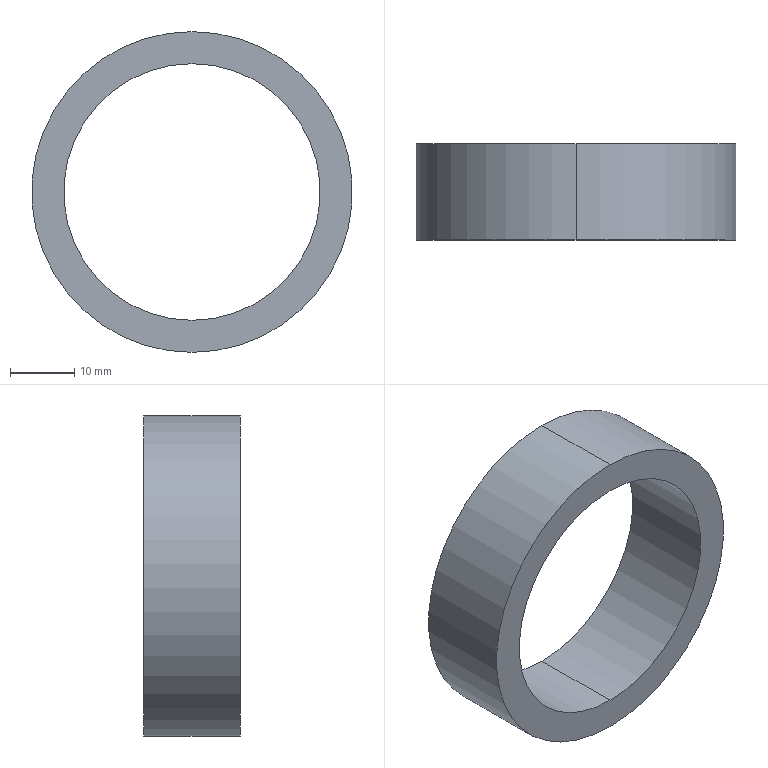Part | SolidWorks | features BaseBody 1 | 1 solid | 6 faces | box 50 x 15 x 50 mm | volume 10603 mm3 | cylinder 4 | plane 2 | commonest cylinder face diameters 40 x2 50 x2
STEP:
#1=CARTESIAN_POINT('',(0.,15.,-25.));
#2=VERTEX_POINT('',#1);
#3=CARTESIAN_POINT('',(0.,15.,25.));
#4=VERTEX_POINT('',#3);
#5=CARTESIAN_POINT('',(0.,15.,0.));
#6=DIRECTION('',(0.,-1.,0.));
#7=DIRECTION('',(0.,0.,-1.));
#8=AXIS2_PLACEMENT_3D('',#5,#6,#7);
#9=CIRCLE('',#8,25.);
#10=EDGE_CURVE('',#2,#4,#9,.T.);
#11=ORIENTED_EDGE('',*,*,#10,.T.);
#12=CARTESIAN_POINT('',(0.,0.,25.));
#13=VERTEX_POINT('',#12);
#14=CARTESIAN_POINT('',(0.,15.,25.));
#15=DIRECTION('',(0.,-1.,0.));
#16=VECTOR('',#15,1000.);
#17=LINE('',#14,#16);
#18=EDGE_CURVE('',#4,#13,#17,.T.);
#19=ORIENTED_EDGE('',*,*,#18,.T.);
#20=CARTESIAN_POINT('',(0.,0.,-25.));
#21=VERTEX_POINT('',#20);
#22=CARTESIAN_POINT('',(0.,0.,0.));
#23=DIRECTION('',(0.,1.,0.));
#24=DIRECTION('',(0.,0.,-1.));
#25=AXIS2_PLACEMENT_3D('',#22,#23,#24);
#26=CIRCLE('',#25,25.);
#27=EDGE_CURVE('',#13,#21,#26,.T.);
#28=ORIENTED_EDGE('',*,*,#27,.T.);
#29=CARTESIAN_POINT('',(0.,15.,-25.));
#30=DIRECTION('',(0.,-1.,0.));
#31=VECTOR('',#30,1000.);
#32=LINE('',#29,#31);
#33=EDGE_CURVE('',#2,#21,#32,.T.);
#34=ORIENTED_EDGE('',*,*,#33,.F.);
#35=EDGE_LOOP('',(#11,#19,#28,#34));
#36=FACE_OUTER_BOUND('',#35,.T.);
#37=CARTESIAN_POINT('',(0.,15.,0.));
#38=DIRECTION('',(0.,-1.,0.));
#39=DIRECTION('',(0.,0.,-1.));
#40=AXIS2_PLACEMENT_3D('',#37,#38,#39);
#41=CYLINDRICAL_SURFACE('',#40,25.);
#42=ADVANCED_FACE('',(#36),#41,.T.);
#43=CARTESIAN_POINT('',(0.,15.,20.));
#44=VERTEX_POINT('',#43);
#45=CARTESIAN_POINT('',(0.,15.,-20.));
#46=VERTEX_POINT('',#45);
#47=CARTESIAN_POINT('',(0.,15.,0.));
#48=DIRECTION('',(0.,-1.,0.));
#49=DIRECTION('',(0.,0.,-1.));
#50=AXIS2_PLACEMENT_3D('',#47,#48,#49);
#51=CIRCLE('',#50,20.);
#52=EDGE_CURVE('',#44,#46,#51,.T.);
#53=ORIENTED_EDGE('',*,*,#52,.F.);
#54=CARTESIAN_POINT('',(0.,0.,20.));
#55=VERTEX_POINT('',#54);
#56=CARTESIAN_POINT('',(0.,15.,20.));
#57=DIRECTION('',(0.,-1.,0.));
#58=VECTOR('',#57,1000.);
#59=LINE('',#56,#58);
#60=EDGE_CURVE('',#44,#55,#59,.T.);
#61=ORIENTED_EDGE('',*,*,#60,.T.);
#62=CARTESIAN_POINT('',(0.,0.,-20.));
#63=VERTEX_POINT('',#62);
#64=CARTESIAN_POINT('',(0.,0.,0.));
#65=DIRECTION('',(0.,-1.,0.));
#66=DIRECTION('',(0.,0.,-1.));
#67=AXIS2_PLACEMENT_3D('',#64,#65,#66);
#68=CIRCLE('',#67,20.);
#69=EDGE_CURVE('',#55,#63,#68,.T.);
#70=ORIENTED_EDGE('',*,*,#69,.T.);
#71=CARTESIAN_POINT('',(0.,15.,-20.));
#72=DIRECTION('',(0.,-1.,0.));
#73=VECTOR('',#72,1000.);
#74=LINE('',#71,#73);
#75=EDGE_CURVE('',#46,#63,#74,.T.);
#76=ORIENTED_EDGE('',*,*,#75,.F.);
#77=EDGE_LOOP('',(#53,#61,#70,#76));
#78=FACE_OUTER_BOUND('',#77,.T.);
#79=CARTESIAN_POINT('',(0.,15.,0.));
#80=DIRECTION('',(0.,-1.,0.));
#81=DIRECTION('',(0.,0.,-1.));
#82=AXIS2_PLACEMENT_3D('',#79,#80,#81);
#83=CYLINDRICAL_SURFACE('',#82,20.);
#84=ADVANCED_FACE('',(#78),#83,.F.);
#85=ORIENTED_EDGE('',*,*,#18,.F.);
#86=CARTESIAN_POINT('',(0.,15.,0.));
#87=DIRECTION('',(0.,-1.,0.));
#88=DIRECTION('',(0.,0.,-1.));
#89=AXIS2_PLACEMENT_3D('',#86,#87,#88);
#90=CIRCLE('',#89,25.);
#91=EDGE_CURVE('',#4,#2,#90,.T.);
#92=ORIENTED_EDGE('',*,*,#91,.T.);
#93=ORIENTED_EDGE('',*,*,#33,.T.);
#94=CARTESIAN_POINT('',(0.,0.,0.));
#95=DIRECTION('',(0.,1.,0.));
#96=DIRECTION('',(0.,0.,-1.));
#97=AXIS2_PLACEMENT_3D('',#94,#95,#96);
#98=CIRCLE('',#97,25.);
#99=EDGE_CURVE('',#21,#13,#98,.T.);
#100=ORIENTED_EDGE('',*,*,#99,.T.);
#101=EDGE_LOOP('',(#85,#92,#93,#100));
#102=FACE_OUTER_BOUND('',#101,.T.);
#103=CARTESIAN_POINT('',(0.,15.,0.));
#104=DIRECTION('',(0.,-1.,0.));
#105=DIRECTION('',(0.,0.,-1.));
#106=AXIS2_PLACEMENT_3D('',#103,#104,#105);
#107=CYLINDRICAL_SURFACE('',#106,25.);
#108=ADVANCED_FACE('',(#102),#107,.T.);
#109=CARTESIAN_POINT('',(0.,0.,0.));
#110=DIRECTION('',(0.,-1.,0.));
#111=DIRECTION('',(0.,0.,-1.));
#112=AXIS2_PLACEMENT_3D('',#109,#110,#111);
#113=CIRCLE('',#112,20.);
#114=EDGE_CURVE('',#63,#55,#113,.T.);
#115=ORIENTED_EDGE('',*,*,#114,.F.);
#116=ORIENTED_EDGE('',*,*,#69,.F.);
#117=EDGE_LOOP('',(#115,#116));
#118=FACE_BOUND('',#117,.T.);
#119=ORIENTED_EDGE('',*,*,#99,.F.);
#120=ORIENTED_EDGE('',*,*,#27,.F.);
#121=EDGE_LOOP('',(#119,#120));
#122=FACE_OUTER_BOUND('',#121,.T.);
#123=CARTESIAN_POINT('',(0.,0.,0.));
#124=DIRECTION('',(0.,1.,0.));
#125=DIRECTION('',(0.,0.,1.));
#126=AXIS2_PLACEMENT_3D('',#123,#124,#125);
#127=PLANE('',#126);
#128=ADVANCED_FACE('',(#118,#122),#127,.F.);
#129=CARTESIAN_POINT('',(0.,15.,0.));
#130=DIRECTION('',(0.,-1.,0.));
#131=DIRECTION('',(0.,0.,-1.));
#132=AXIS2_PLACEMENT_3D('',#129,#130,#131);
#133=CIRCLE('',#132,20.);
#134=EDGE_CURVE('',#46,#44,#133,.T.);
#135=ORIENTED_EDGE('',*,*,#134,.T.);
#136=ORIENTED_EDGE('',*,*,#52,.T.);
#137=EDGE_LOOP('',(#135,#136));
#138=FACE_BOUND('',#137,.T.);
#139=ORIENTED_EDGE('',*,*,#10,.F.);
#140=ORIENTED_EDGE('',*,*,#91,.F.);
#141=EDGE_LOOP('',(#139,#140));
#142=FACE_OUTER_BOUND('',#141,.T.);
#143=CARTESIAN_POINT('',(0.,15.,0.));
#144=DIRECTION('',(0.,1.,0.));
#145=DIRECTION('',(0.,0.,1.));
#146=AXIS2_PLACEMENT_3D('',#143,#144,#145);
#147=PLANE('',#146);
#148=ADVANCED_FACE('',(#138,#142),#147,.T.);
#149=ORIENTED_EDGE('',*,*,#60,.F.);
#150=ORIENTED_EDGE('',*,*,#134,.F.);
#151=ORIENTED_EDGE('',*,*,#75,.T.);
#152=ORIENTED_EDGE('',*,*,#114,.T.);
#153=EDGE_LOOP('',(#149,#150,#151,#152));
#154=FACE_OUTER_BOUND('',#153,.T.);
#155=CARTESIAN_POINT('',(0.,15.,0.));
#156=DIRECTION('',(0.,-1.,0.));
#157=DIRECTION('',(0.,0.,-1.));
#158=AXIS2_PLACEMENT_3D('',#155,#156,#157);
#159=CYLINDRICAL_SURFACE('',#158,20.);
#160=ADVANCED_FACE('',(#154),#159,.F.);
#161=CLOSED_SHELL('',(#42,#84,#108,#128,#148,#160));
#162=MANIFOLD_SOLID_BREP('',#161);
#163=CARTESIAN_POINT('',(0.,0.,0.));
#164=DIRECTION('',(0.,0.,1.));
#165=DIRECTION('',(1.,0.,0.));
#166=AXIS2_PLACEMENT_3D('',#163,#164,#165);
#167=(LENGTH_UNIT()NAMED_UNIT(*)SI_UNIT(.MILLI.,.METRE.));
#168=UNCERTAINTY_MEASURE_WITH_UNIT(LENGTH_MEASURE(0.00001),#167,'','');
#169=(NAMED_UNIT(*)PLANE_ANGLE_UNIT()SI_UNIT($,.RADIAN.));
#170=(NAMED_UNIT(*)SI_UNIT($,.STERADIAN.)SOLID_ANGLE_UNIT());
#171=(GEOMETRIC_REPRESENTATION_CONTEXT(3)GLOBAL_UNCERTAINTY_ASSIGNED_CONTEXT((#168))GLOBAL_UNIT_ASSIGNED_CONTEXT((#167,#169,#170))REPRESENTATION_CONTEXT('',''));
#172=ADVANCED_BREP_SHAPE_REPRESENTATION('',(#162,#166),#171);